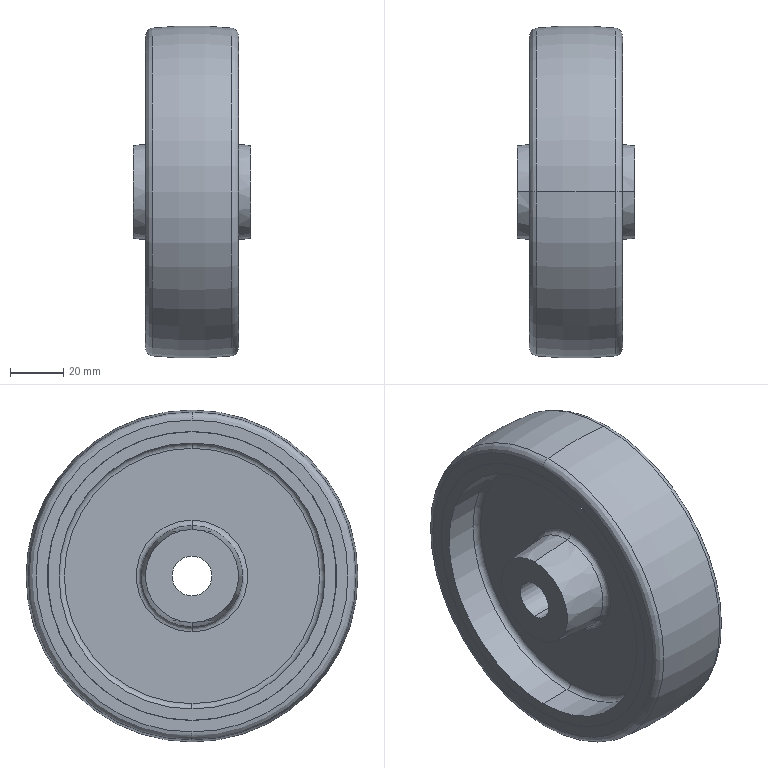Part | STEP file | Frame_top | 1 solid | 42 faces | box 44 x 125 x 125 mm | volume 224779 mm3 | cylinder 14 | torus 12 | plane 10 | cone 4 | other 2 | commonest cylinder face diameters 100 x4 108.535 x4 108.735 x4 15 x2